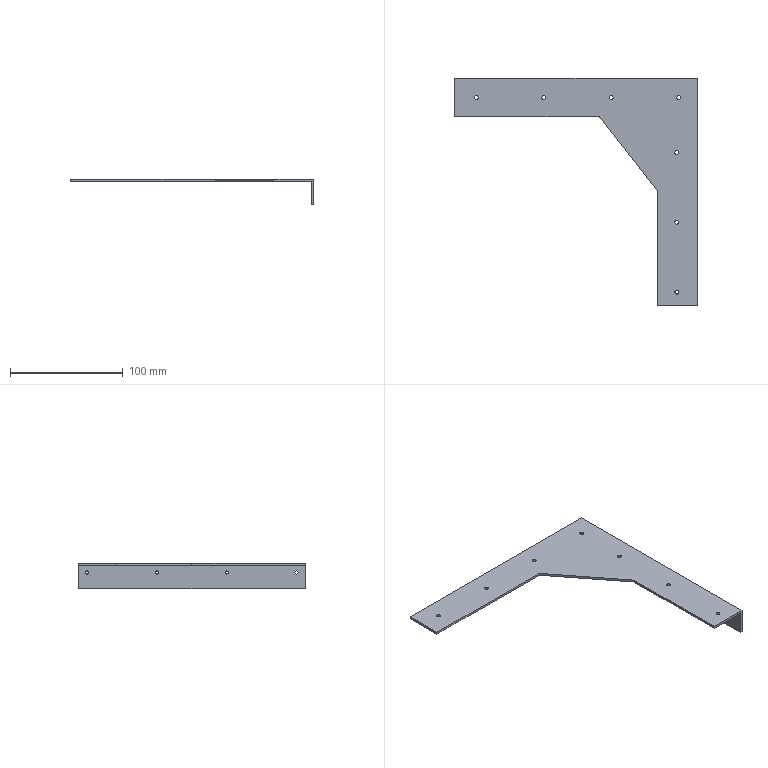Part | SolidWorks | features BaseBody 1 | 1 solid | 33 faces | box 215.539 x 201.719 x 23.05 mm | volume 38142 mm3 | cylinder 22 | plane 11 | commonest cylinder face diameters 3.455 x14 2.781 x8
STEP:
#1=CARTESIAN_POINT('',(-96.681,91.929,0.));
#2=VERTEX_POINT('',#1);
#3=CARTESIAN_POINT('',(-100.136,91.929,0.));
#4=VERTEX_POINT('',#3);
#5=CARTESIAN_POINT('',(-98.408,91.929,0.));
#6=DIRECTION('',(0.,0.,-1.));
#7=DIRECTION('',(-1.,0.,0.));
#8=AXIS2_PLACEMENT_3D('',#5,#6,#7);
#9=CIRCLE('',#8,1.728);
#10=EDGE_CURVE('',#2,#4,#9,.T.);
#11=ORIENTED_EDGE('',*,*,#10,.F.);
#12=CARTESIAN_POINT('',(-96.681,91.929,-2.));
#13=VERTEX_POINT('',#12);
#14=CARTESIAN_POINT('',(-96.681,91.929,-2.));
#15=DIRECTION('',(0.,0.,-1.));
#16=VECTOR('',#15,1000.);
#17=LINE('',#14,#16);
#18=EDGE_CURVE('',#2,#13,#17,.T.);
#19=ORIENTED_EDGE('',*,*,#18,.T.);
#20=CARTESIAN_POINT('',(-100.136,91.929,-2.));
#21=VERTEX_POINT('',#20);
#22=CARTESIAN_POINT('',(-98.408,91.929,-2.));
#23=DIRECTION('',(0.,0.,1.));
#24=DIRECTION('',(-1.,0.,0.));
#25=AXIS2_PLACEMENT_3D('',#22,#23,#24);
#26=CIRCLE('',#25,1.728);
#27=EDGE_CURVE('',#21,#13,#26,.T.);
#28=ORIENTED_EDGE('',*,*,#27,.F.);
#29=CARTESIAN_POINT('',(-100.136,91.929,-2.));
#30=DIRECTION('',(0.,0.,-1.));
#31=VECTOR('',#30,1000.);
#32=LINE('',#29,#31);
#33=EDGE_CURVE('',#4,#21,#32,.T.);
#34=ORIENTED_EDGE('',*,*,#33,.F.);
#35=EDGE_LOOP('',(#11,#19,#28,#34));
#36=FACE_OUTER_BOUND('',#35,.T.);
#37=CARTESIAN_POINT('',(-98.408,91.929,-2.));
#38=DIRECTION('',(0.,0.,-1.));
#39=DIRECTION('',(-1.,0.,0.));
#40=AXIS2_PLACEMENT_3D('',#37,#38,#39);
#41=CYLINDRICAL_SURFACE('',#40,1.728);
#42=ADVANCED_FACE('',(#36),#41,.F.);
#43=CARTESIAN_POINT('',(-36.681,91.929,0.));
#44=VERTEX_POINT('',#43);
#45=CARTESIAN_POINT('',(-40.136,91.929,0.));
#46=VERTEX_POINT('',#45);
#47=CARTESIAN_POINT('',(-38.408,91.929,0.));
#48=DIRECTION('',(0.,0.,-1.));
#49=DIRECTION('',(-1.,0.,0.));
#50=AXIS2_PLACEMENT_3D('',#47,#48,#49);
#51=CIRCLE('',#50,1.728);
#52=EDGE_CURVE('',#44,#46,#51,.T.);
#53=ORIENTED_EDGE('',*,*,#52,.F.);
#54=CARTESIAN_POINT('',(-36.681,91.929,-2.));
#55=VERTEX_POINT('',#54);
#56=CARTESIAN_POINT('',(-36.681,91.929,-2.));
#57=DIRECTION('',(0.,0.,-1.));
#58=VECTOR('',#57,1000.);
#59=LINE('',#56,#58);
#60=EDGE_CURVE('',#44,#55,#59,.T.);
#61=ORIENTED_EDGE('',*,*,#60,.T.);
#62=CARTESIAN_POINT('',(-40.136,91.929,-2.));
#63=VERTEX_POINT('',#62);
#64=CARTESIAN_POINT('',(-38.408,91.929,-2.));
#65=DIRECTION('',(0.,0.,1.));
#66=DIRECTION('',(-1.,0.,0.));
#67=AXIS2_PLACEMENT_3D('',#64,#65,#66);
#68=CIRCLE('',#67,1.728);
#69=EDGE_CURVE('',#63,#55,#68,.T.);
#70=ORIENTED_EDGE('',*,*,#69,.F.);
#71=CARTESIAN_POINT('',(-40.136,91.929,-2.));
#72=DIRECTION('',(0.,0.,-1.));
#73=VECTOR('',#72,1000.);
#74=LINE('',#71,#73);
#75=EDGE_CURVE('',#46,#63,#74,.T.);
#76=ORIENTED_EDGE('',*,*,#75,.F.);
#77=EDGE_LOOP('',(#53,#61,#70,#76));
#78=FACE_OUTER_BOUND('',#77,.T.);
#79=CARTESIAN_POINT('',(-38.408,91.929,-2.));
#80=DIRECTION('',(0.,0.,-1.));
#81=DIRECTION('',(-1.,0.,0.));
#82=AXIS2_PLACEMENT_3D('',#79,#80,#81);
#83=CYLINDRICAL_SURFACE('',#82,1.728);
#84=ADVANCED_FACE('',(#78),#83,.F.);
#85=CARTESIAN_POINT('',(23.319,91.929,0.));
#86=VERTEX_POINT('',#85);
#87=CARTESIAN_POINT('',(19.864,91.929,0.));
#88=VERTEX_POINT('',#87);
#89=CARTESIAN_POINT('',(21.592,91.929,0.));
#90=DIRECTION('',(0.,0.,-1.));
#91=DIRECTION('',(-1.,0.,0.));
#92=AXIS2_PLACEMENT_3D('',#89,#90,#91);
#93=CIRCLE('',#92,1.728);
#94=EDGE_CURVE('',#86,#88,#93,.T.);
#95=ORIENTED_EDGE('',*,*,#94,.F.);
#96=CARTESIAN_POINT('',(23.319,91.929,-2.));
#97=VERTEX_POINT('',#96);
#98=CARTESIAN_POINT('',(23.319,91.929,-2.));
#99=DIRECTION('',(0.,0.,-1.));
#100=VECTOR('',#99,1000.);
#101=LINE('',#98,#100);
#102=EDGE_CURVE('',#86,#97,#101,.T.);
#103=ORIENTED_EDGE('',*,*,#102,.T.);
#104=CARTESIAN_POINT('',(19.864,91.929,-2.));
#105=VERTEX_POINT('',#104);
#106=CARTESIAN_POINT('',(21.592,91.929,-2.));
#107=DIRECTION('',(0.,0.,1.));
#108=DIRECTION('',(-1.,0.,0.));
#109=AXIS2_PLACEMENT_3D('',#106,#107,#108);
#110=CIRCLE('',#109,1.728);
#111=EDGE_CURVE('',#105,#97,#110,.T.);
#112=ORIENTED_EDGE('',*,*,#111,.F.);
#113=CARTESIAN_POINT('',(19.864,91.929,-2.));
#114=DIRECTION('',(0.,0.,-1.));
#115=VECTOR('',#114,1000.);
#116=LINE('',#113,#115);
#117=EDGE_CURVE('',#88,#105,#116,.T.);
#118=ORIENTED_EDGE('',*,*,#117,.F.);
#119=EDGE_LOOP('',(#95,#103,#112,#118));
#120=FACE_OUTER_BOUND('',#119,.T.);
#121=CARTESIAN_POINT('',(21.592,91.929,-2.));
#122=DIRECTION('',(0.,0.,-1.));
#123=DIRECTION('',(-1.,0.,0.));
#124=AXIS2_PLACEMENT_3D('',#121,#122,#123);
#125=CYLINDRICAL_SURFACE('',#124,1.728);
#126=ADVANCED_FACE('',(#120),#125,.F.);
#127=CARTESIAN_POINT('',(81.543,-18.939,0.));
#128=VERTEX_POINT('',#127);
#129=CARTESIAN_POINT('',(78.088,-18.939,0.));
#130=VERTEX_POINT('',#129);
#131=CARTESIAN_POINT('',(79.815,-18.939,0.));
#132=DIRECTION('',(0.,0.,-1.));
#133=DIRECTION('',(-1.,0.,0.));
#134=AXIS2_PLACEMENT_3D('',#131,#132,#133);
#135=CIRCLE('',#134,1.728);
#136=EDGE_CURVE('',#128,#130,#135,.T.);
#137=ORIENTED_EDGE('',*,*,#136,.F.);
#138=CARTESIAN_POINT('',(81.543,-18.939,-2.));
#139=VERTEX_POINT('',#138);
#140=CARTESIAN_POINT('',(81.543,-18.939,-2.));
#141=DIRECTION('',(0.,0.,-1.));
#142=VECTOR('',#141,1000.);
#143=LINE('',#140,#142);
#144=EDGE_CURVE('',#128,#139,#143,.T.);
#145=ORIENTED_EDGE('',*,*,#144,.T.);
#146=CARTESIAN_POINT('',(78.088,-18.939,-2.));
#147=VERTEX_POINT('',#146);
#148=CARTESIAN_POINT('',(79.815,-18.939,-2.));
#149=DIRECTION('',(0.,0.,1.));
#150=DIRECTION('',(-1.,0.,0.));
#151=AXIS2_PLACEMENT_3D('',#148,#149,#150);
#152=CIRCLE('',#151,1.728);
#153=EDGE_CURVE('',#147,#139,#152,.T.);
#154=ORIENTED_EDGE('',*,*,#153,.F.);
#155=CARTESIAN_POINT('',(78.088,-18.939,-2.));
#156=DIRECTION('',(0.,0.,-1.));
#157=VECTOR('',#156,1000.);
#158=LINE('',#155,#157);
#159=EDGE_CURVE('',#130,#147,#158,.T.);
#160=ORIENTED_EDGE('',*,*,#159,.F.);
#161=EDGE_LOOP('',(#137,#145,#154,#160));
#162=FACE_OUTER_BOUND('',#161,.T.);
#163=CARTESIAN_POINT('',(79.815,-18.939,-2.));
#164=DIRECTION('',(0.,0.,-1.));
#165=DIRECTION('',(-1.,0.,0.));
#166=AXIS2_PLACEMENT_3D('',#163,#164,#165);
#167=CYLINDRICAL_SURFACE('',#166,1.728);
#168=ADVANCED_FACE('',(#162),#167,.F.);
#169=CARTESIAN_POINT('',(83.319,91.929,0.));
#170=VERTEX_POINT('',#169);
#171=CARTESIAN_POINT('',(79.864,91.929,0.));
#172=VERTEX_POINT('',#171);
#173=CARTESIAN_POINT('',(81.592,91.929,0.));
#174=DIRECTION('',(0.,0.,-1.));
#175=DIRECTION('',(-1.,0.,0.));
#176=AXIS2_PLACEMENT_3D('',#173,#174,#175);
#177=CIRCLE('',#176,1.728);
#178=EDGE_CURVE('',#170,#172,#177,.T.);
#179=ORIENTED_EDGE('',*,*,#178,.F.);
#180=CARTESIAN_POINT('',(83.319,91.929,-2.));
#181=VERTEX_POINT('',#180);
#182=CARTESIAN_POINT('',(83.319,91.929,-2.));
#183=DIRECTION('',(0.,0.,-1.));
#184=VECTOR('',#183,1000.);
#185=LINE('',#182,#184);
#186=EDGE_CURVE('',#170,#181,#185,.T.);
#187=ORIENTED_EDGE('',*,*,#186,.T.);
#188=CARTESIAN_POINT('',(79.864,91.929,-2.));
#189=VERTEX_POINT('',#188);
#190=CARTESIAN_POINT('',(81.592,91.929,-2.));
#191=DIRECTION('',(0.,0.,1.));
#192=DIRECTION('',(-1.,0.,0.));
#193=AXIS2_PLACEMENT_3D('',#190,#191,#192);
#194=CIRCLE('',#193,1.728);
#195=EDGE_CURVE('',#189,#181,#194,.T.);
#196=ORIENTED_EDGE('',*,*,#195,.F.);
#197=CARTESIAN_POINT('',(79.864,91.929,-2.));
#198=DIRECTION('',(0.,0.,-1.));
#199=VECTOR('',#198,1000.);
#200=LINE('',#197,#199);
#201=EDGE_CURVE('',#172,#189,#200,.T.);
#202=ORIENTED_EDGE('',*,*,#201,.F.);
#203=EDGE_LOOP('',(#179,#187,#196,#202));
#204=FACE_OUTER_BOUND('',#203,.T.);
#205=CARTESIAN_POINT('',(81.592,91.929,-2.));
#206=DIRECTION('',(0.,0.,-1.));
#207=DIRECTION('',(-1.,0.,0.));
#208=AXIS2_PLACEMENT_3D('',#205,#206,#207);
#209=CYLINDRICAL_SURFACE('',#208,1.728);
#210=ADVANCED_FACE('',(#204),#209,.F.);
#211=CARTESIAN_POINT('',(81.543,43.061,0.));
#212=VERTEX_POINT('',#211);
#213=CARTESIAN_POINT('',(78.088,43.061,0.));
#214=VERTEX_POINT('',#213);
#215=CARTESIAN_POINT('',(79.815,43.061,0.));
#216=DIRECTION('',(0.,0.,-1.));
#217=DIRECTION('',(-1.,0.,0.));
#218=AXIS2_PLACEMENT_3D('',#215,#216,#217);
#219=CIRCLE('',#218,1.728);
#220=EDGE_CURVE('',#212,#214,#219,.T.);
#221=ORIENTED_EDGE('',*,*,#220,.F.);
#222=CARTESIAN_POINT('',(81.543,43.061,-2.));
#223=VERTEX_POINT('',#222);
#224=CARTESIAN_POINT('',(81.543,43.061,-2.));
#225=DIRECTION('',(0.,0.,-1.));
#226=VECTOR('',#225,1000.);
#227=LINE('',#224,#226);
#228=EDGE_CURVE('',#212,#223,#227,.T.);
#229=ORIENTED_EDGE('',*,*,#228,.T.);
#230=CARTESIAN_POINT('',(78.088,43.061,-2.));
#231=VERTEX_POINT('',#230);
#232=CARTESIAN_POINT('',(79.815,43.061,-2.));
#233=DIRECTION('',(0.,0.,1.));
#234=DIRECTION('',(-1.,0.,0.));
#235=AXIS2_PLACEMENT_3D('',#232,#233,#234);
#236=CIRCLE('',#235,1.728);
#237=EDGE_CURVE('',#231,#223,#236,.T.);
#238=ORIENTED_EDGE('',*,*,#237,.F.);
#239=CARTESIAN_POINT('',(78.088,43.061,-2.));
#240=DIRECTION('',(0.,0.,-1.));
#241=VECTOR('',#240,1000.);
#242=LINE('',#239,#241);
#243=EDGE_CURVE('',#214,#231,#242,.T.);
#244=ORIENTED_EDGE('',*,*,#243,.F.);
#245=EDGE_LOOP('',(#221,#229,#238,#244));
#246=FACE_OUTER_BOUND('',#245,.T.);
#247=CARTESIAN_POINT('',(79.815,43.061,-2.));
#248=DIRECTION('',(0.,0.,-1.));
#249=DIRECTION('',(-1.,0.,0.));
#250=AXIS2_PLACEMENT_3D('',#247,#248,#249);
#251=CYLINDRICAL_SURFACE('',#250,1.728);
#252=ADVANCED_FACE('',(#246),#251,.F.);
#253=CARTESIAN_POINT('',(81.543,-80.939,0.));
#254=VERTEX_POINT('',#253);
#255=CARTESIAN_POINT('',(78.088,-80.939,0.));
#256=VERTEX_POINT('',#255);
#257=CARTESIAN_POINT('',(79.815,-80.939,0.));
#258=DIRECTION('',(0.,0.,-1.));
#259=DIRECTION('',(-1.,0.,0.));
#260=AXIS2_PLACEMENT_3D('',#257,#258,#259);
#261=CIRCLE('',#260,1.728);
#262=EDGE_CURVE('',#254,#256,#261,.T.);
#263=ORIENTED_EDGE('',*,*,#262,.F.);
#264=CARTESIAN_POINT('',(81.543,-80.939,-2.));
#265=VERTEX_POINT('',#264);
#266=CARTESIAN_POINT('',(81.543,-80.939,-2.));
#267=DIRECTION('',(0.,0.,-1.));
#268=VECTOR('',#267,1000.);
#269=LINE('',#266,#268);
#270=EDGE_CURVE('',#254,#265,#269,.T.);
#271=ORIENTED_EDGE('',*,*,#270,.T.);
#272=CARTESIAN_POINT('',(78.088,-80.939,-2.));
#273=VERTEX_POINT('',#272);
#274=CARTESIAN_POINT('',(79.815,-80.939,-2.));
#275=DIRECTION('',(0.,0.,1.));
#276=DIRECTION('',(-1.,0.,0.));
#277=AXIS2_PLACEMENT_3D('',#274,#275,#276);
#278=CIRCLE('',#277,1.728);
#279=EDGE_CURVE('',#273,#265,#278,.T.);
#280=ORIENTED_EDGE('',*,*,#279,.F.);
#281=CARTESIAN_POINT('',(78.088,-80.939,-2.));
#282=DIRECTION('',(0.,0.,-1.));
#283=VECTOR('',#282,1000.);
#284=LINE('',#281,#283);
#285=EDGE_CURVE('',#256,#273,#284,.T.);
#286=ORIENTED_EDGE('',*,*,#285,.F.);
#287=EDGE_LOOP('',(#263,#271,#280,#286));
#288=FACE_OUTER_BOUND('',#287,.T.);
#289=CARTESIAN_POINT('',(79.815,-80.939,-2.));
#290=DIRECTION('',(0.,0.,-1.));
#291=DIRECTION('',(-1.,0.,0.));
#292=AXIS2_PLACEMENT_3D('',#289,#290,#291);
#293=CYLINDRICAL_SURFACE('',#292,1.728);
#294=ADVANCED_FACE('',(#288),#293,.F.);
#295=CARTESIAN_POINT('',(98.025,101.141,-7.031));
#296=VERTEX_POINT('',#295);
#297=CARTESIAN_POINT('',(98.025,101.141,-9.812));
#298=VERTEX_POINT('',#297);
#299=CARTESIAN_POINT('',(98.025,101.141,-8.421));
#300=DIRECTION('',(1.,0.,0.));
#301=DIRECTION('',(0.,0.,1.));
#302=AXIS2_PLACEMENT_3D('',#299,#300,#301);
#303=CIRCLE('',#302,1.39);
#304=EDGE_CURVE('',#296,#298,#303,.T.);
#305=ORIENTED_EDGE('',*,*,#304,.T.);
#306=CARTESIAN_POINT('',(96.025,101.141,-9.812));
#307=VERTEX_POINT('',#306);
#308=CARTESIAN_POINT('',(96.025,101.141,-9.812));
#309=DIRECTION('',(-1.,0.,0.));
#310=VECTOR('',#309,1000.);
#311=LINE('',#308,#310);
#312=EDGE_CURVE('',#298,#307,#311,.T.);
#313=ORIENTED_EDGE('',*,*,#312,.T.);
#314=CARTESIAN_POINT('',(96.025,101.141,-7.031));
#315=VERTEX_POINT('',#314);
#316=CARTESIAN_POINT('',(96.025,101.141,-8.421));
#317=DIRECTION('',(-1.,0.,0.));
#318=DIRECTION('',(0.,0.,1.));
#319=AXIS2_PLACEMENT_3D('',#316,#317,#318);
#320=CIRCLE('',#319,1.39);
#321=EDGE_CURVE('',#307,#315,#320,.T.);
#322=ORIENTED_EDGE('',*,*,#321,.T.);
#323=CARTESIAN_POINT('',(96.025,101.141,-7.031));
#324=DIRECTION('',(-1.,0.,0.));
#325=VECTOR('',#324,1000.);
#326=LINE('',#323,#325);
#327=EDGE_CURVE('',#296,#315,#326,.T.);
#328=ORIENTED_EDGE('',*,*,#327,.F.);
#329=EDGE_LOOP('',(#305,#313,#322,#328));
#330=FACE_OUTER_BOUND('',#329,.T.);
#331=CARTESIAN_POINT('',(96.025,101.141,-8.421));
#332=DIRECTION('',(-1.,0.,0.));
#333=DIRECTION('',(0.,0.,1.));
#334=AXIS2_PLACEMENT_3D('',#331,#332,#333);
#335=CYLINDRICAL_SURFACE('',#334,1.39);
#336=ADVANCED_FACE('',(#330),#335,.F.);
#337=CARTESIAN_POINT('',(98.025,-84.859,-7.031));
#338=VERTEX_POINT('',#337);
#339=CARTESIAN_POINT('',(98.025,-84.859,-9.812));
#340=VERTEX_POINT('',#339);
#341=CARTESIAN_POINT('',(98.025,-84.859,-8.421));
#342=DIRECTION('',(1.,0.,0.));
#343=DIRECTION('',(0.,0.,1.));
#344=AXIS2_PLACEMENT_3D('',#341,#342,#343);
#345=CIRCLE('',#344,1.39);
#346=EDGE_CURVE('',#338,#340,#345,.T.);
#347=ORIENTED_EDGE('',*,*,#346,.T.);
#348=CARTESIAN_POINT('',(96.025,-84.859,-9.812));
#349=VERTEX_POINT('',#348);
#350=CARTESIAN_POINT('',(96.025,-84.859,-9.812));
#351=DIRECTION('',(-1.,0.,0.));
#352=VECTOR('',#351,1000.);
#353=LINE('',#350,#352);
#354=EDGE_CURVE('',#340,#349,#353,.T.);
#355=ORIENTED_EDGE('',*,*,#354,.T.);
#356=CARTESIAN_POINT('',(96.025,-84.859,-7.031));
#357=VERTEX_POINT('',#356);
#358=CARTESIAN_POINT('',(96.025,-84.859,-8.421));
#359=DIRECTION('',(-1.,0.,0.));
#360=DIRECTION('',(0.,0.,1.));
#361=AXIS2_PLACEMENT_3D('',#358,#359,#360);
#362=CIRCLE('',#361,1.39);
#363=EDGE_CURVE('',#349,#357,#362,.T.);
#364=ORIENTED_EDGE('',*,*,#363,.T.);
#365=CARTESIAN_POINT('',(96.025,-84.859,-7.031));
#366=DIRECTION('',(-1.,0.,0.));
#367=VECTOR('',#366,1000.);
#368=LINE('',#365,#367);
#369=EDGE_CURVE('',#338,#357,#368,.T.);
#370=ORIENTED_EDGE('',*,*,#369,.F.);
#371=EDGE_LOOP('',(#347,#355,#364,#370));
#372=FACE_OUTER_BOUND('',#371,.T.);
#373=CARTESIAN_POINT('',(96.025,-84.859,-8.421));
#374=DIRECTION('',(-1.,0.,0.));
#375=DIRECTION('',(0.,0.,1.));
#376=AXIS2_PLACEMENT_3D('',#373,#374,#375);
#377=CYLINDRICAL_SURFACE('',#376,1.39);
#378=ADVANCED_FACE('',(#372),#377,.F.);
#379=CARTESIAN_POINT('',(98.025,-24.25,-8.421));
#380=VERTEX_POINT('',#379);
#381=CARTESIAN_POINT('',(98.025,-21.469,-8.421));
#382=VERTEX_POINT('',#381);
#383=CARTESIAN_POINT('',(98.025,-22.859,-8.421));
#384=DIRECTION('',(1.,0.,0.));
#385=DIRECTION('',(0.,-1.,0.));
#386=AXIS2_PLACEMENT_3D('',#383,#384,#385);
#387=CIRCLE('',#386,1.39);
#388=EDGE_CURVE('',#380,#382,#387,.T.);
#389=ORIENTED_EDGE('',*,*,#388,.T.);
#390=CARTESIAN_POINT('',(96.025,-21.469,-8.421));
#391=VERTEX_POINT('',#390);
#392=CARTESIAN_POINT('',(96.025,-21.469,-8.421));
#393=DIRECTION('',(-1.,0.,0.));
#394=VECTOR('',#393,1000.);
#395=LINE('',#392,#394);
#396=EDGE_CURVE('',#382,#391,#395,.T.);
#397=ORIENTED_EDGE('',*,*,#396,.T.);
#398=CARTESIAN_POINT('',(96.025,-24.25,-8.421));
#399=VERTEX_POINT('',#398);
#400=CARTESIAN_POINT('',(96.025,-22.859,-8.421));
#401=DIRECTION('',(-1.,0.,0.));
#402=DIRECTION('',(0.,-1.,0.));
#403=AXIS2_PLACEMENT_3D('',#400,#401,#402);
#404=CIRCLE('',#403,1.39);
#405=EDGE_CURVE('',#391,#399,#404,.T.);
#406=ORIENTED_EDGE('',*,*,#405,.T.);
#407=CARTESIAN_POINT('',(96.025,-24.25,-8.421));
#408=DIRECTION('',(-1.,0.,0.));
#409=VECTOR('',#408,1000.);
#410=LINE('',#407,#409);
#411=EDGE_CURVE('',#380,#399,#410,.T.);
#412=ORIENTED_EDGE('',*,*,#411,.F.);
#413=EDGE_LOOP('',(#389,#397,#406,#412));
#414=FACE_OUTER_BOUND('',#413,.T.);
#415=CARTESIAN_POINT('',(96.025,-22.859,-8.421));
#416=DIRECTION('',(-1.,0.,0.));
#417=DIRECTION('',(0.,-1.,0.));
#418=AXIS2_PLACEMENT_3D('',#415,#416,#417);
#419=CYLINDRICAL_SURFACE('',#418,1.39);
#420=ADVANCED_FACE('',(#414),#419,.F.);
#421=CARTESIAN_POINT('',(98.025,37.75,-8.421));
#422=VERTEX_POINT('',#421);
#423=CARTESIAN_POINT('',(98.025,40.531,-8.421));
#424=VERTEX_POINT('',#423);
#425=CARTESIAN_POINT('',(98.025,39.141,-8.421));
#426=DIRECTION('',(1.,0.,0.));
#427=DIRECTION('',(0.,-1.,0.));
#428=AXIS2_PLACEMENT_3D('',#425,#426,#427);
#429=CIRCLE('',#428,1.39);
#430=EDGE_CURVE('',#422,#424,#429,.T.);
#431=ORIENTED_EDGE('',*,*,#430,.T.);
#432=CARTESIAN_POINT('',(96.025,40.531,-8.421));
#433=VERTEX_POINT('',#432);
#434=CARTESIAN_POINT('',(96.025,40.531,-8.421));
#435=DIRECTION('',(-1.,0.,0.));
#436=VECTOR('',#435,1000.);
#437=LINE('',#434,#436);
#438=EDGE_CURVE('',#424,#433,#437,.T.);
#439=ORIENTED_EDGE('',*,*,#438,.T.);
#440=CARTESIAN_POINT('',(96.025,37.75,-8.421));
#441=VERTEX_POINT('',#440);
#442=CARTESIAN_POINT('',(96.025,39.141,-8.421));
#443=DIRECTION('',(-1.,0.,0.));
#444=DIRECTION('',(0.,-1.,0.));
#445=AXIS2_PLACEMENT_3D('',#442,#443,#444);
#446=CIRCLE('',#445,1.39);
#447=EDGE_CURVE('',#433,#441,#446,.T.);
#448=ORIENTED_EDGE('',*,*,#447,.T.);
#449=CARTESIAN_POINT('',(96.025,37.75,-8.421));
#450=DIRECTION('',(-1.,0.,0.));
#451=VECTOR('',#450,1000.);
#452=LINE('',#449,#451);
#453=EDGE_CURVE('',#422,#441,#452,.T.);
#454=ORIENTED_EDGE('',*,*,#453,.F.);
#455=EDGE_LOOP('',(#431,#439,#448,#454));
#456=FACE_OUTER_BOUND('',#455,.T.);
#457=CARTESIAN_POINT('',(96.025,39.141,-8.421));
#458=DIRECTION('',(-1.,0.,0.));
#459=DIRECTION('',(0.,-1.,0.));
#460=AXIS2_PLACEMENT_3D('',#457,#458,#459);
#461=CYLINDRICAL_SURFACE('',#460,1.39);
#462=ADVANCED_FACE('',(#456),#461,.F.);
#463=CARTESIAN_POINT('',(-98.408,91.929,0.));
#464=DIRECTION('',(0.,0.,-1.));
#465=DIRECTION('',(-1.,0.,0.));
#466=AXIS2_PLACEMENT_3D('',#463,#464,#465);
#467=CIRCLE('',#466,1.728);
#468=EDGE_CURVE('',#4,#2,#467,.T.);
#469=ORIENTED_EDGE('',*,*,#468,.T.);
#470=ORIENTED_EDGE('',*,*,#10,.T.);
#471=EDGE_LOOP('',(#469,#470));
#472=FACE_BOUND('',#471,.T.);
#473=CARTESIAN_POINT('',(-38.408,91.929,0.));
#474=DIRECTION('',(0.,0.,-1.));
#475=DIRECTION('',(-1.,0.,0.));
#476=AXIS2_PLACEMENT_3D('',#473,#474,#475);
#477=CIRCLE('',#476,1.728);
#478=EDGE_CURVE('',#46,#44,#477,.T.);
#479=ORIENTED_EDGE('',*,*,#478,.T.);
#480=ORIENTED_EDGE('',*,*,#52,.T.);
#481=EDGE_LOOP('',(#479,#480));
#482=FACE_BOUND('',#481,.T.);
#483=CARTESIAN_POINT('',(21.592,91.929,0.));
#484=DIRECTION('',(0.,0.,-1.));
#485=DIRECTION('',(-1.,0.,0.));
#486=AXIS2_PLACEMENT_3D('',#483,#484,#485);
#487=CIRCLE('',#486,1.728);
#488=EDGE_CURVE('',#88,#86,#487,.T.);
#489=ORIENTED_EDGE('',*,*,#488,.T.);
#490=ORIENTED_EDGE('',*,*,#94,.T.);
#491=EDGE_LOOP('',(#489,#490));
#492=FACE_BOUND('',#491,.T.);
#493=CARTESIAN_POINT('',(79.815,-18.939,0.));
#494=DIRECTION('',(0.,0.,-1.));
#495=DIRECTION('',(-1.,0.,0.));
#496=AXIS2_PLACEMENT_3D('',#493,#494,#495);
#497=CIRCLE('',#496,1.728);
#498=EDGE_CURVE('',#130,#128,#497,.T.);
#499=ORIENTED_EDGE('',*,*,#498,.T.);
#500=ORIENTED_EDGE('',*,*,#136,.T.);
#501=EDGE_LOOP('',(#499,#500));
#502=FACE_BOUND('',#501,.T.);
#503=CARTESIAN_POINT('',(81.592,91.929,0.));
#504=DIRECTION('',(0.,0.,-1.));
#505=DIRECTION('',(-1.,0.,0.));
#506=AXIS2_PLACEMENT_3D('',#503,#504,#505);
#507=CIRCLE('',#506,1.728);
#508=EDGE_CURVE('',#172,#170,#507,.T.);
#509=ORIENTED_EDGE('',*,*,#508,.T.);
#510=ORIENTED_EDGE('',*,*,#178,.T.);
#511=EDGE_LOOP('',(#509,#510));
#512=FACE_BOUND('',#511,.T.);
#513=CARTESIAN_POINT('',(79.815,43.061,0.));
#514=DIRECTION('',(0.,0.,-1.));
#515=DIRECTION('',(-1.,0.,0.));
#516=AXIS2_PLACEMENT_3D('',#513,#514,#515);
#517=CIRCLE('',#516,1.728);
#518=EDGE_CURVE('',#214,#212,#517,.T.);
#519=ORIENTED_EDGE('',*,*,#518,.T.);
#520=ORIENTED_EDGE('',*,*,#220,.T.);
#521=EDGE_LOOP('',(#519,#520));
#522=FACE_BOUND('',#521,.T.);
#523=CARTESIAN_POINT('',(79.815,-80.939,0.));
#524=DIRECTION('',(0.,0.,-1.));
#525=DIRECTION('',(-1.,0.,0.));
#526=AXIS2_PLACEMENT_3D('',#523,#524,#525);
#527=CIRCLE('',#526,1.728);
#528=EDGE_CURVE('',#256,#254,#527,.T.);
#529=ORIENTED_EDGE('',*,*,#528,.T.);
#530=ORIENTED_EDGE('',*,*,#262,.T.);
#531=EDGE_LOOP('',(#529,#530));
#532=FACE_BOUND('',#531,.T.);
#533=CARTESIAN_POINT('',(10.832,74.984,0.));
#534=VERTEX_POINT('',#533);
#535=CARTESIAN_POINT('',(63.089,8.12,0.));
#536=VERTEX_POINT('',#535);
#537=CARTESIAN_POINT('',(10.832,74.984,0.));
#538=DIRECTION('',(0.6158,-0.7879,0.));
#539=VECTOR('',#538,1000.);
#540=LINE('',#537,#539);
#541=EDGE_CURVE('',#534,#536,#540,.T.);
#542=ORIENTED_EDGE('',*,*,#541,.T.);
#543=CARTESIAN_POINT('',(63.089,-92.846,0.));
#544=VERTEX_POINT('',#543);
#545=CARTESIAN_POINT('',(63.089,8.014,0.));
#546=DIRECTION('',(0.,-1.,0.));
#547=VECTOR('',#546,1000.);
#548=LINE('',#545,#547);
#549=EDGE_CURVE('',#536,#544,#548,.T.);
#550=ORIENTED_EDGE('',*,*,#549,.T.);
#551=CARTESIAN_POINT('',(98.025,-92.846,0.));
#552=VERTEX_POINT('',#551);
#553=CARTESIAN_POINT('',(-9.744,-92.846,0.));
#554=DIRECTION('',(1.,0.,0.));
#555=VECTOR('',#554,1000.);
#556=LINE('',#553,#555);
#557=EDGE_CURVE('',#544,#552,#556,.T.);
#558=ORIENTED_EDGE('',*,*,#557,.T.);
#559=CARTESIAN_POINT('',(98.025,108.873,0.));
#560=VERTEX_POINT('',#559);
#561=CARTESIAN_POINT('',(98.025,8.014,0.));
#562=DIRECTION('',(0.,1.,0.));
#563=VECTOR('',#562,1000.);
#564=LINE('',#561,#563);
#565=EDGE_CURVE('',#552,#560,#564,.T.);
#566=ORIENTED_EDGE('',*,*,#565,.T.);
#567=CARTESIAN_POINT('',(-117.514,108.873,0.));
#568=VERTEX_POINT('',#567);
#569=CARTESIAN_POINT('',(-9.744,108.873,0.));
#570=DIRECTION('',(-1.,0.,0.));
#571=VECTOR('',#570,1000.);
#572=LINE('',#569,#571);
#573=EDGE_CURVE('',#560,#568,#572,.T.);
#574=ORIENTED_EDGE('',*,*,#573,.T.);
#575=CARTESIAN_POINT('',(-117.514,74.984,0.));
#576=VERTEX_POINT('',#575);
#577=CARTESIAN_POINT('',(-117.514,8.014,0.));
#578=DIRECTION('',(0.,-1.,0.));
#579=VECTOR('',#578,1000.);
#580=LINE('',#577,#579);
#581=EDGE_CURVE('',#568,#576,#580,.T.);
#582=ORIENTED_EDGE('',*,*,#581,.T.);
#583=CARTESIAN_POINT('',(-9.744,74.984,0.));
#584=DIRECTION('',(1.,0.,0.));
#585=VECTOR('',#584,1000.);
#586=LINE('',#583,#585);
#587=EDGE_CURVE('',#576,#534,#586,.T.);
#588=ORIENTED_EDGE('',*,*,#587,.T.);
#589=EDGE_LOOP('',(#542,#550,#558,#566,#574,#582,#588));
#590=FACE_OUTER_BOUND('',#589,.T.);
#591=CARTESIAN_POINT('',(-9.744,8.014,0.));
#592=DIRECTION('',(0.,0.,1.));
#593=DIRECTION('',(1.,0.,0.));
#594=AXIS2_PLACEMENT_3D('',#591,#592,#593);
#595=PLANE('',#594);
#596=ADVANCED_FACE('',(#472,#482,#492,#502,#512,#522,#532,#590),#595,.T.);
#597=ORIENTED_EDGE('',*,*,#18,.F.);
#598=ORIENTED_EDGE('',*,*,#468,.F.);
#599=ORIENTED_EDGE('',*,*,#33,.T.);
#600=CARTESIAN_POINT('',(-98.408,91.929,-2.));
#601=DIRECTION('',(0.,0.,1.));
#602=DIRECTION('',(-1.,0.,0.));
#603=AXIS2_PLACEMENT_3D('',#600,#601,#602);
#604=CIRCLE('',#603,1.728);
#605=EDGE_CURVE('',#13,#21,#604,.T.);
#606=ORIENTED_EDGE('',*,*,#605,.F.);
#607=EDGE_LOOP('',(#597,#598,#599,#606));
#608=FACE_OUTER_BOUND('',#607,.T.);
#609=CARTESIAN_POINT('',(-98.408,91.929,-2.));
#610=DIRECTION('',(0.,0.,-1.));
#611=DIRECTION('',(-1.,0.,0.));
#612=AXIS2_PLACEMENT_3D('',#609,#610,#611);
#613=CYLINDRICAL_SURFACE('',#612,1.728);
#614=ADVANCED_FACE('',(#608),#613,.F.);
#615=ORIENTED_EDGE('',*,*,#60,.F.);
#616=ORIENTED_EDGE('',*,*,#478,.F.);
#617=ORIENTED_EDGE('',*,*,#75,.T.);
#618=CARTESIAN_POINT('',(-38.408,91.929,-2.));
#619=DIRECTION('',(0.,0.,1.));
#620=DIRECTION('',(-1.,0.,0.));
#621=AXIS2_PLACEMENT_3D('',#618,#619,#620);
#622=CIRCLE('',#621,1.728);
#623=EDGE_CURVE('',#55,#63,#622,.T.);
#624=ORIENTED_EDGE('',*,*,#623,.F.);
#625=EDGE_LOOP('',(#615,#616,#617,#624));
#626=FACE_OUTER_BOUND('',#625,.T.);
#627=CARTESIAN_POINT('',(-38.408,91.929,-2.));
#628=DIRECTION('',(0.,0.,-1.));
#629=DIRECTION('',(-1.,0.,0.));
#630=AXIS2_PLACEMENT_3D('',#627,#628,#629);
#631=CYLINDRICAL_SURFACE('',#630,1.728);
#632=ADVANCED_FACE('',(#626),#631,.F.);
#633=ORIENTED_EDGE('',*,*,#102,.F.);
#634=ORIENTED_EDGE('',*,*,#488,.F.);
#635=ORIENTED_EDGE('',*,*,#117,.T.);
#636=CARTESIAN_POINT('',(21.592,91.929,-2.));
#637=DIRECTION('',(0.,0.,1.));
#638=DIRECTION('',(-1.,0.,0.));
#639=AXIS2_PLACEMENT_3D('',#636,#637,#638);
#640=CIRCLE('',#639,1.728);
#641=EDGE_CURVE('',#97,#105,#640,.T.);
#642=ORIENTED_EDGE('',*,*,#641,.F.);
#643=EDGE_LOOP('',(#633,#634,#635,#642));
#644=FACE_OUTER_BOUND('',#643,.T.);
#645=CARTESIAN_POINT('',(21.592,91.929,-2.));
#646=DIRECTION('',(0.,0.,-1.));
#647=DIRECTION('',(-1.,0.,0.));
#648=AXIS2_PLACEMENT_3D('',#645,#646,#647);
#649=CYLINDRICAL_SURFACE('',#648,1.728);
#650=ADVANCED_FACE('',(#644),#649,.F.);
#651=ORIENTED_EDGE('',*,*,#144,.F.);
#652=ORIENTED_EDGE('',*,*,#498,.F.);
#653=ORIENTED_EDGE('',*,*,#159,.T.);
#654=CARTESIAN_POINT('',(79.815,-18.939,-2.));
#655=DIRECTION('',(0.,0.,1.));
#656=DIRECTION('',(-1.,0.,0.));
#657=AXIS2_PLACEMENT_3D('',#654,#655,#656);
#658=CIRCLE('',#657,1.728);
#659=EDGE_CURVE('',#139,#147,#658,.T.);
#660=ORIENTED_EDGE('',*,*,#659,.F.);
#661=EDGE_LOOP('',(#651,#652,#653,#660));
#662=FACE_OUTER_BOUND('',#661,.T.);
#663=CARTESIAN_POINT('',(79.815,-18.939,-2.));
#664=DIRECTION('',(0.,0.,-1.));
#665=DIRECTION('',(-1.,0.,0.));
#666=AXIS2_PLACEMENT_3D('',#663,#664,#665);
#667=CYLINDRICAL_SURFACE('',#666,1.728);
#668=ADVANCED_FACE('',(#662),#667,.F.);
#669=ORIENTED_EDGE('',*,*,#186,.F.);
#670=ORIENTED_EDGE('',*,*,#508,.F.);
#671=ORIENTED_EDGE('',*,*,#201,.T.);
#672=CARTESIAN_POINT('',(81.592,91.929,-2.));
#673=DIRECTION('',(0.,0.,1.));
#674=DIRECTION('',(-1.,0.,0.));
#675=AXIS2_PLACEMENT_3D('',#672,#673,#674);
#676=CIRCLE('',#675,1.728);
#677=EDGE_CURVE('',#181,#189,#676,.T.);
#678=ORIENTED_EDGE('',*,*,#677,.F.);
#679=EDGE_LOOP('',(#669,#670,#671,#678));
#680=FACE_OUTER_BOUND('',#679,.T.);
#681=CARTESIAN_POINT('',(81.592,91.929,-2.));
#682=DIRECTION('',(0.,0.,-1.));
#683=DIRECTION('',(-1.,0.,0.));
#684=AXIS2_PLACEMENT_3D('',#681,#682,#683);
#685=CYLINDRICAL_SURFACE('',#684,1.728);
#686=ADVANCED_FACE('',(#680),#685,.F.);
#687=ORIENTED_EDGE('',*,*,#228,.F.);
#688=ORIENTED_EDGE('',*,*,#518,.F.);
#689=ORIENTED_EDGE('',*,*,#243,.T.);
#690=CARTESIAN_POINT('',(79.815,43.061,-2.));
#691=DIRECTION('',(0.,0.,1.));
#692=DIRECTION('',(-1.,0.,0.));
#693=AXIS2_PLACEMENT_3D('',#690,#691,#692);
#694=CIRCLE('',#693,1.728);
#695=EDGE_CURVE('',#223,#231,#694,.T.);
#696=ORIENTED_EDGE('',*,*,#695,.F.);
#697=EDGE_LOOP('',(#687,#688,#689,#696));
#698=FACE_OUTER_BOUND('',#697,.T.);
#699=CARTESIAN_POINT('',(79.815,43.061,-2.));
#700=DIRECTION('',(0.,0.,-1.));
#701=DIRECTION('',(-1.,0.,0.));
#702=AXIS2_PLACEMENT_3D('',#699,#700,#701);
#703=CYLINDRICAL_SURFACE('',#702,1.728);
#704=ADVANCED_FACE('',(#698),#703,.F.);
#705=ORIENTED_EDGE('',*,*,#270,.F.);
#706=ORIENTED_EDGE('',*,*,#528,.F.);
#707=ORIENTED_EDGE('',*,*,#285,.T.);
#708=CARTESIAN_POINT('',(79.815,-80.939,-2.));
#709=DIRECTION('',(0.,0.,1.));
#710=DIRECTION('',(-1.,0.,0.));
#711=AXIS2_PLACEMENT_3D('',#708,#709,#710);
#712=CIRCLE('',#711,1.728);
#713=EDGE_CURVE('',#265,#273,#712,.T.);
#714=ORIENTED_EDGE('',*,*,#713,.F.);
#715=EDGE_LOOP('',(#705,#706,#707,#714));
#716=FACE_OUTER_BOUND('',#715,.T.);
#717=CARTESIAN_POINT('',(79.815,-80.939,-2.));
#718=DIRECTION('',(0.,0.,-1.));
#719=DIRECTION('',(-1.,0.,0.));
#720=AXIS2_PLACEMENT_3D('',#717,#718,#719);
#721=CYLINDRICAL_SURFACE('',#720,1.728);
#722=ADVANCED_FACE('',(#716),#721,.F.);
#723=CARTESIAN_POINT('',(63.089,8.12,-2.));
#724=VERTEX_POINT('',#723);
#725=CARTESIAN_POINT('',(63.089,8.12,0.));
#726=DIRECTION('',(0.,0.,1.));
#727=VECTOR('',#726,1000.);
#728=LINE('',#725,#727);
#729=EDGE_CURVE('',#724,#536,#728,.T.);
#730=ORIENTED_EDGE('',*,*,#729,.F.);
#731=CARTESIAN_POINT('',(63.089,-92.846,-2.));
#732=VERTEX_POINT('',#731);
#733=CARTESIAN_POINT('',(63.089,8.12,-2.));
#734=DIRECTION('',(0.,1.,0.));
#735=VECTOR('',#734,1000.);
#736=LINE('',#733,#735);
#737=EDGE_CURVE('',#732,#724,#736,.T.);
#738=ORIENTED_EDGE('',*,*,#737,.F.);
#739=CARTESIAN_POINT('',(63.089,-92.846,0.));
#740=DIRECTION('',(0.,0.,-1.));
#741=VECTOR('',#740,1000.);
#742=LINE('',#739,#741);
#743=EDGE_CURVE('',#544,#732,#742,.T.);
#744=ORIENTED_EDGE('',*,*,#743,.F.);
#745=ORIENTED_EDGE('',*,*,#549,.F.);
#746=EDGE_LOOP('',(#730,#738,#744,#745));
#747=FACE_OUTER_BOUND('',#746,.T.);
#748=CARTESIAN_POINT('',(63.089,8.12,0.));
#749=DIRECTION('',(1.,0.,0.));
#750=DIRECTION('',(0.,1.,0.));
#751=AXIS2_PLACEMENT_3D('',#748,#749,#750);
#752=PLANE('',#751);
#753=ADVANCED_FACE('',(#747),#752,.F.);
#754=CARTESIAN_POINT('',(10.832,74.984,-2.));
#755=VERTEX_POINT('',#754);
#756=CARTESIAN_POINT('',(10.832,74.984,0.));
#757=DIRECTION('',(0.,0.,1.));
#758=VECTOR('',#757,1000.);
#759=LINE('',#756,#758);
#760=EDGE_CURVE('',#755,#534,#759,.T.);
#761=ORIENTED_EDGE('',*,*,#760,.F.);
#762=CARTESIAN_POINT('',(10.832,74.984,-2.));
#763=DIRECTION('',(-0.6158,0.7879,0.));
#764=VECTOR('',#763,1000.);
#765=LINE('',#762,#764);
#766=EDGE_CURVE('',#724,#755,#765,.T.);
#767=ORIENTED_EDGE('',*,*,#766,.F.);
#768=ORIENTED_EDGE('',*,*,#729,.T.);
#769=ORIENTED_EDGE('',*,*,#541,.F.);
#770=EDGE_LOOP('',(#761,#767,#768,#769));
#771=FACE_OUTER_BOUND('',#770,.T.);
#772=CARTESIAN_POINT('',(10.832,74.984,0.));
#773=DIRECTION('',(0.7879,0.6158,0.));
#774=DIRECTION('',(-0.6158,0.7879,0.));
#775=AXIS2_PLACEMENT_3D('',#772,#773,#774);
#776=PLANE('',#775);
#777=ADVANCED_FACE('',(#771),#776,.F.);
#778=CARTESIAN_POINT('',(-117.514,74.984,-2.));
#779=VERTEX_POINT('',#778);
#780=CARTESIAN_POINT('',(-117.514,74.984,0.));
#781=DIRECTION('',(0.,0.,1.));
#782=VECTOR('',#781,1000.);
#783=LINE('',#780,#782);
#784=EDGE_CURVE('',#779,#576,#783,.T.);
#785=ORIENTED_EDGE('',*,*,#784,.F.);
#786=CARTESIAN_POINT('',(-117.514,74.984,-2.));
#787=DIRECTION('',(-1.,0.,0.));
#788=VECTOR('',#787,1000.);
#789=LINE('',#786,#788);
#790=EDGE_CURVE('',#755,#779,#789,.T.);
#791=ORIENTED_EDGE('',*,*,#790,.F.);
#792=ORIENTED_EDGE('',*,*,#760,.T.);
#793=ORIENTED_EDGE('',*,*,#587,.F.);
#794=EDGE_LOOP('',(#785,#791,#792,#793));
#795=FACE_OUTER_BOUND('',#794,.T.);
#796=CARTESIAN_POINT('',(-117.514,74.984,0.));
#797=DIRECTION('',(0.,1.,0.));
#798=DIRECTION('',(-1.,0.,0.));
#799=AXIS2_PLACEMENT_3D('',#796,#797,#798);
#800=PLANE('',#799);
#801=ADVANCED_FACE('',(#795),#800,.F.);
#802=CARTESIAN_POINT('',(-117.514,108.873,-2.));
#803=VERTEX_POINT('',#802);
#804=CARTESIAN_POINT('',(-117.514,108.873,0.));
#805=DIRECTION('',(0.,0.,1.));
#806=VECTOR('',#805,1000.);
#807=LINE('',#804,#806);
#808=EDGE_CURVE('',#803,#568,#807,.T.);
#809=ORIENTED_EDGE('',*,*,#808,.F.);
#810=CARTESIAN_POINT('',(-117.514,108.873,-2.));
#811=DIRECTION('',(0.,1.,0.));
#812=VECTOR('',#811,1000.);
#813=LINE('',#810,#812);
#814=EDGE_CURVE('',#779,#803,#813,.T.);
#815=ORIENTED_EDGE('',*,*,#814,.F.);
#816=ORIENTED_EDGE('',*,*,#784,.T.);
#817=ORIENTED_EDGE('',*,*,#581,.F.);
#818=EDGE_LOOP('',(#809,#815,#816,#817));
#819=FACE_OUTER_BOUND('',#818,.T.);
#820=CARTESIAN_POINT('',(-117.514,108.873,0.));
#821=DIRECTION('',(1.,0.,0.));
#822=DIRECTION('',(0.,0.,-1.));
#823=AXIS2_PLACEMENT_3D('',#820,#821,#822);
#824=PLANE('',#823);
#825=ADVANCED_FACE('',(#819),#824,.F.);
#826=CARTESIAN_POINT('',(98.025,108.873,-23.05));
#827=VERTEX_POINT('',#826);
#828=CARTESIAN_POINT('',(98.025,108.873,0.));
#829=DIRECTION('',(0.,0.,1.));
#830=VECTOR('',#829,1000.);
#831=LINE('',#828,#830);
#832=EDGE_CURVE('',#827,#560,#831,.T.);
#833=ORIENTED_EDGE('',*,*,#832,.F.);
#834=CARTESIAN_POINT('',(96.025,108.873,-23.05));
#835=VERTEX_POINT('',#834);
#836=CARTESIAN_POINT('',(98.025,108.873,-23.05));
#837=DIRECTION('',(1.,0.,0.));
#838=VECTOR('',#837,1000.);
#839=LINE('',#836,#838);
#840=EDGE_CURVE('',#835,#827,#839,.T.);
#841=ORIENTED_EDGE('',*,*,#840,.F.);
#842=CARTESIAN_POINT('',(96.025,108.873,-2.));
#843=VERTEX_POINT('',#842);
#844=CARTESIAN_POINT('',(96.025,108.873,0.));
#845=DIRECTION('',(0.,0.,-1.));
#846=VECTOR('',#845,1000.);
#847=LINE('',#844,#846);
#848=EDGE_CURVE('',#843,#835,#847,.T.);
#849=ORIENTED_EDGE('',*,*,#848,.F.);
#850=CARTESIAN_POINT('',(98.025,108.873,-2.));
#851=DIRECTION('',(1.,0.,0.));
#852=VECTOR('',#851,1000.);
#853=LINE('',#850,#852);
#854=EDGE_CURVE('',#803,#843,#853,.T.);
#855=ORIENTED_EDGE('',*,*,#854,.F.);
#856=ORIENTED_EDGE('',*,*,#808,.T.);
#857=ORIENTED_EDGE('',*,*,#573,.F.);
#858=EDGE_LOOP('',(#833,#841,#849,#855,#856,#857));
#859=FACE_OUTER_BOUND('',#858,.T.);
#860=CARTESIAN_POINT('',(98.025,108.873,0.));
#861=DIRECTION('',(0.,-1.,0.));
#862=DIRECTION('',(1.,0.,0.));
#863=AXIS2_PLACEMENT_3D('',#860,#861,#862);
#864=PLANE('',#863);
#865=ADVANCED_FACE('',(#859),#864,.F.);
#866=ORIENTED_EDGE('',*,*,#304,.F.);
#867=CARTESIAN_POINT('',(98.025,101.141,-8.421));
#868=DIRECTION('',(1.,0.,0.));
#869=DIRECTION('',(0.,0.,1.));
#870=AXIS2_PLACEMENT_3D('',#867,#868,#869);
#871=CIRCLE('',#870,1.39);
#872=EDGE_CURVE('',#298,#296,#871,.T.);
#873=ORIENTED_EDGE('',*,*,#872,.F.);
#874=EDGE_LOOP('',(#866,#873));
#875=FACE_BOUND('',#874,.T.);
#876=ORIENTED_EDGE('',*,*,#346,.F.);
#877=CARTESIAN_POINT('',(98.025,-84.859,-8.421));
#878=DIRECTION('',(1.,0.,0.));
#879=DIRECTION('',(0.,0.,1.));
#880=AXIS2_PLACEMENT_3D('',#877,#878,#879);
#881=CIRCLE('',#880,1.39);
#882=EDGE_CURVE('',#340,#338,#881,.T.);
#883=ORIENTED_EDGE('',*,*,#882,.F.);
#884=EDGE_LOOP('',(#876,#883));
#885=FACE_BOUND('',#884,.T.);
#886=ORIENTED_EDGE('',*,*,#388,.F.);
#887=CARTESIAN_POINT('',(98.025,-22.859,-8.421));
#888=DIRECTION('',(1.,0.,0.));
#889=DIRECTION('',(0.,-1.,0.));
#890=AXIS2_PLACEMENT_3D('',#887,#888,#889);
#891=CIRCLE('',#890,1.39);
#892=EDGE_CURVE('',#382,#380,#891,.T.);
#893=ORIENTED_EDGE('',*,*,#892,.F.);
#894=EDGE_LOOP('',(#886,#893));
#895=FACE_BOUND('',#894,.T.);
#896=ORIENTED_EDGE('',*,*,#430,.F.);
#897=CARTESIAN_POINT('',(98.025,39.141,-8.421));
#898=DIRECTION('',(1.,0.,0.));
#899=DIRECTION('',(0.,-1.,0.));
#900=AXIS2_PLACEMENT_3D('',#897,#898,#899);
#901=CIRCLE('',#900,1.39);
#902=EDGE_CURVE('',#424,#422,#901,.T.);
#903=ORIENTED_EDGE('',*,*,#902,.F.);
#904=EDGE_LOOP('',(#896,#903));
#905=FACE_BOUND('',#904,.T.);
#906=CARTESIAN_POINT('',(98.025,-92.846,-23.05));
#907=VERTEX_POINT('',#906);
#908=CARTESIAN_POINT('',(98.025,-92.846,0.));
#909=DIRECTION('',(0.,0.,1.));
#910=VECTOR('',#909,1000.);
#911=LINE('',#908,#910);
#912=EDGE_CURVE('',#907,#552,#911,.T.);
#913=ORIENTED_EDGE('',*,*,#912,.F.);
#914=CARTESIAN_POINT('',(98.025,-92.846,-23.05));
#915=DIRECTION('',(0.,-1.,0.));
#916=VECTOR('',#915,1000.);
#917=LINE('',#914,#916);
#918=EDGE_CURVE('',#827,#907,#917,.T.);
#919=ORIENTED_EDGE('',*,*,#918,.F.);
#920=ORIENTED_EDGE('',*,*,#832,.T.);
#921=ORIENTED_EDGE('',*,*,#565,.F.);
#922=EDGE_LOOP('',(#913,#919,#920,#921));
#923=FACE_OUTER_BOUND('',#922,.T.);
#924=CARTESIAN_POINT('',(98.025,-92.846,0.));
#925=DIRECTION('',(-1.,0.,0.));
#926=DIRECTION('',(0.,-1.,0.));
#927=AXIS2_PLACEMENT_3D('',#924,#925,#926);
#928=PLANE('',#927);
#929=ADVANCED_FACE('',(#875,#885,#895,#905,#923),#928,.F.);
#930=ORIENTED_EDGE('',*,*,#743,.T.);
#931=CARTESIAN_POINT('',(96.025,-92.846,-2.));
#932=VERTEX_POINT('',#931);
#933=CARTESIAN_POINT('',(63.089,-92.846,-2.));
#934=DIRECTION('',(-1.,0.,0.));
#935=VECTOR('',#934,1000.);
#936=LINE('',#933,#935);
#937=EDGE_CURVE('',#932,#732,#936,.T.);
#938=ORIENTED_EDGE('',*,*,#937,.F.);
#939=CARTESIAN_POINT('',(96.025,-92.846,-23.05));
#940=VERTEX_POINT('',#939);
#941=CARTESIAN_POINT('',(96.025,-92.846,0.));
#942=DIRECTION('',(0.,0.,1.));
#943=VECTOR('',#942,1000.);
#944=LINE('',#941,#943);
#945=EDGE_CURVE('',#940,#932,#944,.T.);
#946=ORIENTED_EDGE('',*,*,#945,.F.);
#947=CARTESIAN_POINT('',(63.089,-92.846,-23.05));
#948=DIRECTION('',(-1.,0.,0.));
#949=VECTOR('',#948,1000.);
#950=LINE('',#947,#949);
#951=EDGE_CURVE('',#907,#940,#950,.T.);
#952=ORIENTED_EDGE('',*,*,#951,.F.);
#953=ORIENTED_EDGE('',*,*,#912,.T.);
#954=ORIENTED_EDGE('',*,*,#557,.F.);
#955=EDGE_LOOP('',(#930,#938,#946,#952,#953,#954));
#956=FACE_OUTER_BOUND('',#955,.T.);
#957=CARTESIAN_POINT('',(63.089,-92.846,0.));
#958=DIRECTION('',(0.,1.,0.));
#959=DIRECTION('',(-1.,0.,0.));
#960=AXIS2_PLACEMENT_3D('',#957,#958,#959);
#961=PLANE('',#960);
#962=ADVANCED_FACE('',(#956),#961,.F.);
#963=ORIENTED_EDGE('',*,*,#27,.T.);
#964=ORIENTED_EDGE('',*,*,#605,.T.);
#965=EDGE_LOOP('',(#963,#964));
#966=FACE_BOUND('',#965,.T.);
#967=ORIENTED_EDGE('',*,*,#69,.T.);
#968=ORIENTED_EDGE('',*,*,#623,.T.);
#969=EDGE_LOOP('',(#967,#968));
#970=FACE_BOUND('',#969,.T.);
#971=ORIENTED_EDGE('',*,*,#111,.T.);
#972=ORIENTED_EDGE('',*,*,#641,.T.);
#973=EDGE_LOOP('',(#971,#972));
#974=FACE_BOUND('',#973,.T.);
#975=ORIENTED_EDGE('',*,*,#153,.T.);
#976=ORIENTED_EDGE('',*,*,#659,.T.);
#977=EDGE_LOOP('',(#975,#976));
#978=FACE_BOUND('',#977,.T.);
#979=ORIENTED_EDGE('',*,*,#195,.T.);
#980=ORIENTED_EDGE('',*,*,#677,.T.);
#981=EDGE_LOOP('',(#979,#980));
#982=FACE_BOUND('',#981,.T.);
#983=ORIENTED_EDGE('',*,*,#237,.T.);
#984=ORIENTED_EDGE('',*,*,#695,.T.);
#985=EDGE_LOOP('',(#983,#984));
#986=FACE_BOUND('',#985,.T.);
#987=ORIENTED_EDGE('',*,*,#279,.T.);
#988=ORIENTED_EDGE('',*,*,#713,.T.);
#989=EDGE_LOOP('',(#987,#988));
#990=FACE_BOUND('',#989,.T.);
#991=ORIENTED_EDGE('',*,*,#937,.T.);
#992=ORIENTED_EDGE('',*,*,#737,.T.);
#993=ORIENTED_EDGE('',*,*,#766,.T.);
#994=ORIENTED_EDGE('',*,*,#790,.T.);
#995=ORIENTED_EDGE('',*,*,#814,.T.);
#996=ORIENTED_EDGE('',*,*,#854,.T.);
#997=CARTESIAN_POINT('',(96.025,8.014,-2.));
#998=DIRECTION('',(0.,1.,0.));
#999=VECTOR('',#998,1000.);
#1000=LINE('',#997,#999);
#1001=EDGE_CURVE('',#932,#843,#1000,.T.);
#1002=ORIENTED_EDGE('',*,*,#1001,.F.);
#1003=EDGE_LOOP('',(#991,#992,#993,#994,#995,#996,#1002));
#1004=FACE_OUTER_BOUND('',#1003,.T.);
#1005=CARTESIAN_POINT('',(-9.744,8.014,-2.));
#1006=DIRECTION('',(0.,0.,1.));
#1007=DIRECTION('',(1.,0.,0.));
#1008=AXIS2_PLACEMENT_3D('',#1005,#1006,#1007);
#1009=PLANE('',#1008);
#1010=ADVANCED_FACE('',(#966,#970,#974,#978,#982,#986,#990,#1004),#1009,.F.);
#1011=ORIENTED_EDGE('',*,*,#918,.T.);
#1012=ORIENTED_EDGE('',*,*,#951,.T.);
#1013=CARTESIAN_POINT('',(96.025,8.014,-23.05));
#1014=DIRECTION('',(0.,-1.,0.));
#1015=VECTOR('',#1014,1000.);
#1016=LINE('',#1013,#1015);
#1017=EDGE_CURVE('',#835,#940,#1016,.T.);
#1018=ORIENTED_EDGE('',*,*,#1017,.F.);
#1019=ORIENTED_EDGE('',*,*,#840,.T.);
#1020=EDGE_LOOP('',(#1011,#1012,#1018,#1019));
#1021=FACE_OUTER_BOUND('',#1020,.T.);
#1022=CARTESIAN_POINT('',(97.025,8.014,-23.05));
#1023=DIRECTION('',(0.,0.,1.));
#1024=DIRECTION('',(1.,0.,0.));
#1025=AXIS2_PLACEMENT_3D('',#1022,#1023,#1024);
#1026=PLANE('',#1025);
#1027=ADVANCED_FACE('',(#1021),#1026,.F.);
#1028=CARTESIAN_POINT('',(96.025,101.141,-8.421));
#1029=DIRECTION('',(-1.,0.,0.));
#1030=DIRECTION('',(0.,0.,1.));
#1031=AXIS2_PLACEMENT_3D('',#1028,#1029,#1030);
#1032=CIRCLE('',#1031,1.39);
#1033=EDGE_CURVE('',#315,#307,#1032,.T.);
#1034=ORIENTED_EDGE('',*,*,#1033,.F.);
#1035=ORIENTED_EDGE('',*,*,#321,.F.);
#1036=EDGE_LOOP('',(#1034,#1035));
#1037=FACE_BOUND('',#1036,.T.);
#1038=CARTESIAN_POINT('',(96.025,-84.859,-8.421));
#1039=DIRECTION('',(-1.,0.,0.));
#1040=DIRECTION('',(0.,0.,1.));
#1041=AXIS2_PLACEMENT_3D('',#1038,#1039,#1040);
#1042=CIRCLE('',#1041,1.39);
#1043=EDGE_CURVE('',#357,#349,#1042,.T.);
#1044=ORIENTED_EDGE('',*,*,#1043,.F.);
#1045=ORIENTED_EDGE('',*,*,#363,.F.);
#1046=EDGE_LOOP('',(#1044,#1045));
#1047=FACE_BOUND('',#1046,.T.);
#1048=CARTESIAN_POINT('',(96.025,-22.859,-8.421));
#1049=DIRECTION('',(-1.,0.,0.));
#1050=DIRECTION('',(0.,-1.,0.));
#1051=AXIS2_PLACEMENT_3D('',#1048,#1049,#1050);
#1052=CIRCLE('',#1051,1.39);
#1053=EDGE_CURVE('',#399,#391,#1052,.T.);
#1054=ORIENTED_EDGE('',*,*,#1053,.F.);
#1055=ORIENTED_EDGE('',*,*,#405,.F.);
#1056=EDGE_LOOP('',(#1054,#1055));
#1057=FACE_BOUND('',#1056,.T.);
#1058=CARTESIAN_POINT('',(96.025,39.141,-8.421));
#1059=DIRECTION('',(-1.,0.,0.));
#1060=DIRECTION('',(0.,-1.,0.));
#1061=AXIS2_PLACEMENT_3D('',#1058,#1059,#1060);
#1062=CIRCLE('',#1061,1.39);
#1063=EDGE_CURVE('',#441,#433,#1062,.T.);
#1064=ORIENTED_EDGE('',*,*,#1063,.F.);
#1065=ORIENTED_EDGE('',*,*,#447,.F.);
#1066=EDGE_LOOP('',(#1064,#1065));
#1067=FACE_BOUND('',#1066,.T.);
#1068=ORIENTED_EDGE('',*,*,#848,.T.);
#1069=ORIENTED_EDGE('',*,*,#1017,.T.);
#1070=ORIENTED_EDGE('',*,*,#945,.T.);
#1071=ORIENTED_EDGE('',*,*,#1001,.T.);
#1072=EDGE_LOOP('',(#1068,#1069,#1070,#1071));
#1073=FACE_OUTER_BOUND('',#1072,.T.);
#1074=CARTESIAN_POINT('',(96.025,108.873,-2.));
#1075=DIRECTION('',(1.,0.,0.));
#1076=DIRECTION('',(0.,1.,0.));
#1077=AXIS2_PLACEMENT_3D('',#1074,#1075,#1076);
#1078=PLANE('',#1077);
#1079=ADVANCED_FACE('',(#1037,#1047,#1057,#1067,#1073),#1078,.F.);
#1080=ORIENTED_EDGE('',*,*,#312,.F.);
#1081=ORIENTED_EDGE('',*,*,#872,.T.);
#1082=ORIENTED_EDGE('',*,*,#327,.T.);
#1083=ORIENTED_EDGE('',*,*,#1033,.T.);
#1084=EDGE_LOOP('',(#1080,#1081,#1082,#1083));
#1085=FACE_OUTER_BOUND('',#1084,.T.);
#1086=CARTESIAN_POINT('',(96.025,101.141,-8.421));
#1087=DIRECTION('',(-1.,0.,0.));
#1088=DIRECTION('',(0.,0.,1.));
#1089=AXIS2_PLACEMENT_3D('',#1086,#1087,#1088);
#1090=CYLINDRICAL_SURFACE('',#1089,1.39);
#1091=ADVANCED_FACE('',(#1085),#1090,.F.);
#1092=ORIENTED_EDGE('',*,*,#354,.F.);
#1093=ORIENTED_EDGE('',*,*,#882,.T.);
#1094=ORIENTED_EDGE('',*,*,#369,.T.);
#1095=ORIENTED_EDGE('',*,*,#1043,.T.);
#1096=EDGE_LOOP('',(#1092,#1093,#1094,#1095));
#1097=FACE_OUTER_BOUND('',#1096,.T.);
#1098=CARTESIAN_POINT('',(96.025,-84.859,-8.421));
#1099=DIRECTION('',(-1.,0.,0.));
#1100=DIRECTION('',(0.,0.,1.));
#1101=AXIS2_PLACEMENT_3D('',#1098,#1099,#1100);
#1102=CYLINDRICAL_SURFACE('',#1101,1.39);
#1103=ADVANCED_FACE('',(#1097),#1102,.F.);
#1104=ORIENTED_EDGE('',*,*,#396,.F.);
#1105=ORIENTED_EDGE('',*,*,#892,.T.);
#1106=ORIENTED_EDGE('',*,*,#411,.T.);
#1107=ORIENTED_EDGE('',*,*,#1053,.T.);
#1108=EDGE_LOOP('',(#1104,#1105,#1106,#1107));
#1109=FACE_OUTER_BOUND('',#1108,.T.);
#1110=CARTESIAN_POINT('',(96.025,-22.859,-8.421));
#1111=DIRECTION('',(-1.,0.,0.));
#1112=DIRECTION('',(0.,-1.,0.));
#1113=AXIS2_PLACEMENT_3D('',#1110,#1111,#1112);
#1114=CYLINDRICAL_SURFACE('',#1113,1.39);
#1115=ADVANCED_FACE('',(#1109),#1114,.F.);
#1116=ORIENTED_EDGE('',*,*,#438,.F.);
#1117=ORIENTED_EDGE('',*,*,#902,.T.);
#1118=ORIENTED_EDGE('',*,*,#453,.T.);
#1119=ORIENTED_EDGE('',*,*,#1063,.T.);
#1120=EDGE_LOOP('',(#1116,#1117,#1118,#1119));
#1121=FACE_OUTER_BOUND('',#1120,.T.);
#1122=CARTESIAN_POINT('',(96.025,39.141,-8.421));
#1123=DIRECTION('',(-1.,0.,0.));
#1124=DIRECTION('',(0.,-1.,0.));
#1125=AXIS2_PLACEMENT_3D('',#1122,#1123,#1124);
#1126=CYLINDRICAL_SURFACE('',#1125,1.39);
#1127=ADVANCED_FACE('',(#1121),#1126,.F.);
#1128=CLOSED_SHELL('',(#42,#84,#126,#168,#210,#252,#294,#336,#378,#420,#462,#596,#614,#632,#650,#668,#686,#704,#722,#753,#777,#801,#825,#865,#929,#962,#1010,#1027,#1079,#1091,#1103,#1115,#1127));
#1129=MANIFOLD_SOLID_BREP('',#1128);
#1130=CARTESIAN_POINT('',(0.,0.,0.));
#1131=DIRECTION('',(0.,0.,1.));
#1132=DIRECTION('',(1.,0.,0.));
#1133=AXIS2_PLACEMENT_3D('',#1130,#1131,#1132);
#1134=(LENGTH_UNIT()NAMED_UNIT(*)SI_UNIT(.MILLI.,.METRE.));
#1135=UNCERTAINTY_MEASURE_WITH_UNIT(LENGTH_MEASURE(0.00001),#1134,'','');
#1136=(NAMED_UNIT(*)PLANE_ANGLE_UNIT()SI_UNIT($,.RADIAN.));
#1137=(NAMED_UNIT(*)SI_UNIT($,.STERADIAN.)SOLID_ANGLE_UNIT());
#1138=(GEOMETRIC_REPRESENTATION_CONTEXT(3)GLOBAL_UNCERTAINTY_ASSIGNED_CONTEXT((#1135))GLOBAL_UNIT_ASSIGNED_CONTEXT((#1134,#1136,#1137))REPRESENTATION_CONTEXT('',''));
#1139=ADVANCED_BREP_SHAPE_REPRESENTATION('',(#1129,#1133),#1138);